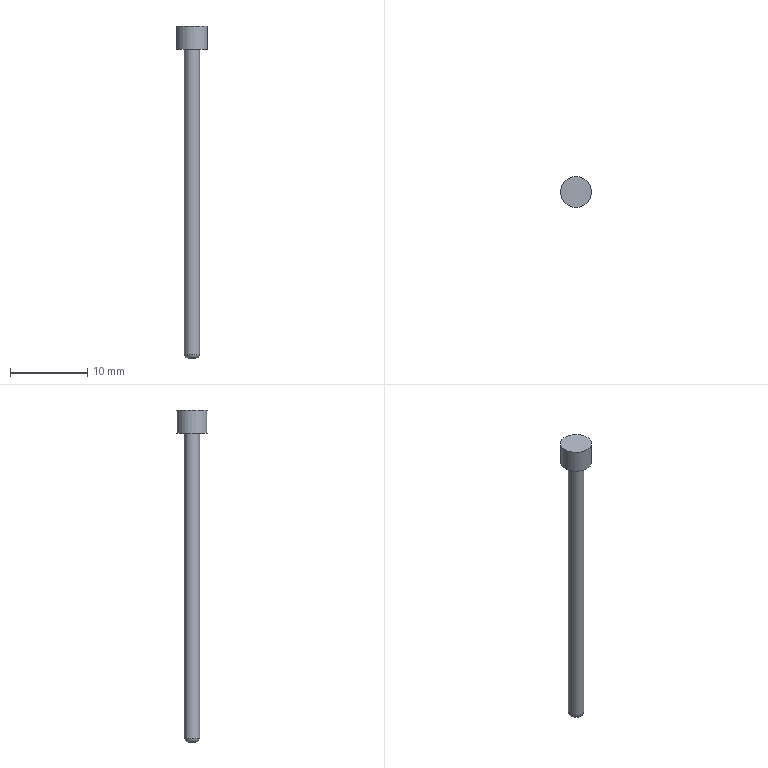Part | NX | features solid 2 | 1 solid | 6 faces | box 4 x 4 x 43 mm | volume 163.063 mm3 | plane 3 | cylinder 2 | torus 1 | commonest cylinder face diameters 2 x1 4 x1
STEP:
#1=CARTESIAN_POINT('',(710.624,-92.983,-11.));
#2=VERTEX_POINT('',#1);
#3=CARTESIAN_POINT('',(711.124,-92.983,-11.));
#4=DIRECTION('',(0.,0.,-1.));
#5=DIRECTION('',(-1.,0.,0.));
#6=AXIS2_PLACEMENT_3D('',#3,#4,#5);
#7=CIRCLE('',#6,0.5);
#8=EDGE_CURVE('',#2,#2,#7,.T.);
#9=ORIENTED_EDGE('',*,*,#8,.T.);
#10=EDGE_LOOP('',(#9));
#11=FACE_BOUND('',#10,.T.);
#12=CARTESIAN_POINT('',(711.124,-92.983,-11.));
#13=DIRECTION('',(0.,0.,-1.));
#14=DIRECTION('',(-1.,0.,0.));
#15=AXIS2_PLACEMENT_3D('',#12,#13,#14);
#16=PLANE('',#15);
#17=ADVANCED_FACE('',(#11),#16,.T.);
#18=CARTESIAN_POINT('',(710.124,-92.983,29.));
#19=VERTEX_POINT('',#18);
#20=CARTESIAN_POINT('',(711.124,-92.983,29.));
#21=DIRECTION('',(0.,0.,-1.));
#22=DIRECTION('',(-1.,0.,0.));
#23=AXIS2_PLACEMENT_3D('',#20,#21,#22);
#24=CIRCLE('',#23,1.);
#25=EDGE_CURVE('',#19,#19,#24,.F.);
#26=ORIENTED_EDGE('',*,*,#25,.F.);
#27=EDGE_LOOP('',(#26));
#28=FACE_BOUND('',#27,.T.);
#29=CARTESIAN_POINT('',(710.124,-92.983,-10.5));
#30=VERTEX_POINT('',#29);
#31=CARTESIAN_POINT('',(711.124,-92.983,-10.5));
#32=DIRECTION('',(0.,0.,-1.));
#33=DIRECTION('',(-1.,0.,0.));
#34=AXIS2_PLACEMENT_3D('',#31,#32,#33);
#35=CIRCLE('',#34,1.);
#36=EDGE_CURVE('',#30,#30,#35,.F.);
#37=ORIENTED_EDGE('',*,*,#36,.T.);
#38=EDGE_LOOP('',(#37));
#39=FACE_BOUND('',#38,.T.);
#40=CARTESIAN_POINT('',(711.124,-92.983,32.));
#41=DIRECTION('',(0.,0.,-1.));
#42=DIRECTION('',(1.,0.,0.));
#43=AXIS2_PLACEMENT_3D('',#40,#41,#42);
#44=CYLINDRICAL_SURFACE('',#43,1.);
#45=ADVANCED_FACE('',(#28,#39),#44,.T.);
#46=ORIENTED_EDGE('',*,*,#8,.F.);
#47=EDGE_LOOP('',(#46));
#48=FACE_BOUND('',#47,.T.);
#49=ORIENTED_EDGE('',*,*,#36,.F.);
#50=EDGE_LOOP('',(#49));
#51=FACE_BOUND('',#50,.T.);
#52=CARTESIAN_POINT('',(711.124,-92.983,-10.5));
#53=DIRECTION('',(0.,0.,-1.));
#54=DIRECTION('',(-1.,0.,0.));
#55=AXIS2_PLACEMENT_3D('',#52,#53,#54);
#56=TOROIDAL_SURFACE('',#55,0.5,0.5);
#57=ADVANCED_FACE('',(#48,#51),#56,.T.);
#58=ORIENTED_EDGE('',*,*,#25,.T.);
#59=EDGE_LOOP('',(#58));
#60=FACE_BOUND('',#59,.T.);
#61=CARTESIAN_POINT('',(713.124,-92.983,29.));
#62=VERTEX_POINT('',#61);
#63=CARTESIAN_POINT('',(711.124,-92.983,29.));
#64=DIRECTION('',(0.,0.,1.));
#65=DIRECTION('',(1.,0.,0.));
#66=AXIS2_PLACEMENT_3D('',#63,#64,#65);
#67=CIRCLE('',#66,2.);
#68=EDGE_CURVE('',#62,#62,#67,.T.);
#69=ORIENTED_EDGE('',*,*,#68,.F.);
#70=EDGE_LOOP('',(#69));
#71=FACE_BOUND('',#70,.T.);
#72=CARTESIAN_POINT('',(711.124,-92.983,29.));
#73=DIRECTION('',(0.,0.,-1.));
#74=DIRECTION('',(-1.,0.,0.));
#75=AXIS2_PLACEMENT_3D('',#72,#73,#74);
#76=PLANE('',#75);
#77=ADVANCED_FACE('',(#60,#71),#76,.T.);
#78=ORIENTED_EDGE('',*,*,#68,.T.);
#79=EDGE_LOOP('',(#78));
#80=FACE_BOUND('',#79,.T.);
#81=CARTESIAN_POINT('',(713.124,-92.983,32.));
#82=VERTEX_POINT('',#81);
#83=CARTESIAN_POINT('',(711.124,-92.983,32.));
#84=DIRECTION('',(0.,0.,-1.));
#85=DIRECTION('',(1.,0.,0.));
#86=AXIS2_PLACEMENT_3D('',#83,#84,#85);
#87=CIRCLE('',#86,2.);
#88=EDGE_CURVE('',#82,#82,#87,.T.);
#89=ORIENTED_EDGE('',*,*,#88,.T.);
#90=EDGE_LOOP('',(#89));
#91=FACE_BOUND('',#90,.T.);
#92=CARTESIAN_POINT('',(711.124,-92.983,32.));
#93=DIRECTION('',(0.,0.,-1.));
#94=DIRECTION('',(1.,0.,0.));
#95=AXIS2_PLACEMENT_3D('',#92,#93,#94);
#96=CYLINDRICAL_SURFACE('',#95,2.);
#97=ADVANCED_FACE('',(#80,#91),#96,.T.);
#98=ORIENTED_EDGE('',*,*,#88,.F.);
#99=EDGE_LOOP('',(#98));
#100=FACE_BOUND('',#99,.T.);
#101=CARTESIAN_POINT('',(711.124,-92.983,32.));
#102=DIRECTION('',(0.,0.,1.));
#103=DIRECTION('',(1.,0.,0.));
#104=AXIS2_PLACEMENT_3D('',#101,#102,#103);
#105=PLANE('',#104);
#106=ADVANCED_FACE('',(#100),#105,.T.);
#107=CLOSED_SHELL('',(#17,#45,#57,#77,#97,#106));
#108=MANIFOLD_SOLID_BREP('',#107);
#109=(LENGTH_UNIT()NAMED_UNIT(*)SI_UNIT(.MILLI.,.METRE.));
#110=UNCERTAINTY_MEASURE_WITH_UNIT(LENGTH_MEASURE(0.00001),#109,'','');
#111=(NAMED_UNIT(*)PLANE_ANGLE_UNIT()SI_UNIT($,.RADIAN.));
#112=(NAMED_UNIT(*)SI_UNIT($,.STERADIAN.)SOLID_ANGLE_UNIT());
#113=(GEOMETRIC_REPRESENTATION_CONTEXT(3)GLOBAL_UNCERTAINTY_ASSIGNED_CONTEXT((#110))GLOBAL_UNIT_ASSIGNED_CONTEXT((#109,#111,#112))REPRESENTATION_CONTEXT('',''));
#114=ADVANCED_BREP_SHAPE_REPRESENTATION('',(#108),#113);